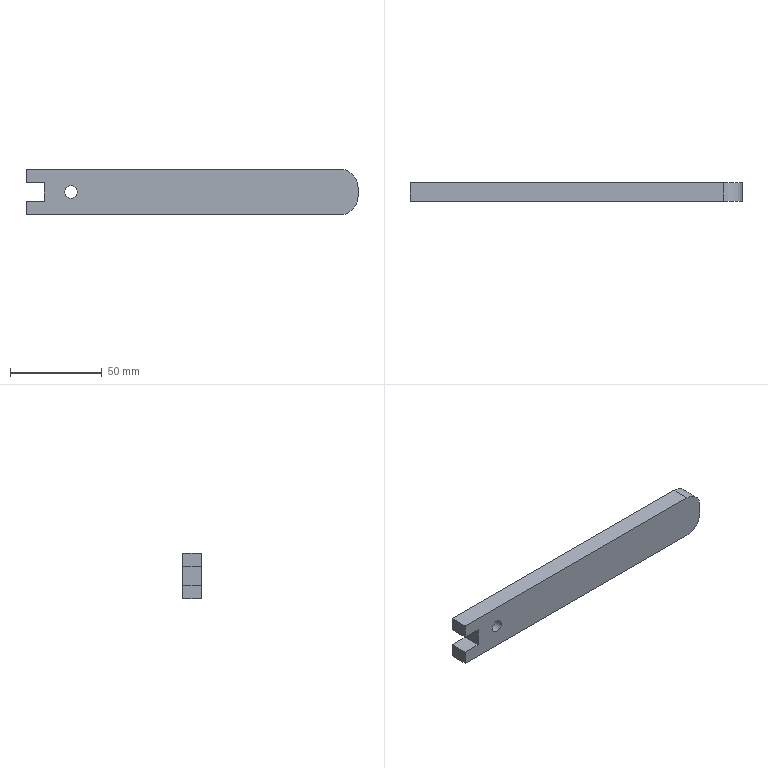Part | NX | features DATUM_CSYS 1, EXTRACT_DATUM_PLANE 1, EXTRUDE 1, SKETCH 1 | 1 solid | 13 faces | box 180.75 x 10 x 25 mm | volume 43395 mm3 | plane 10 | cylinder 3 | commonest cylinder face diameters 20 x2 6.8 x1
STEP:
#1=CARTESIAN_POINT('',(169.25,5.,17.214));
#2=VERTEX_POINT('',#1);
#3=CARTESIAN_POINT('',(169.25,5.,24.714));
#4=VERTEX_POINT('',#3);
#5=CARTESIAN_POINT('',(169.25,5.,17.214));
#6=DIRECTION('',(0.,0.,1.));
#7=VECTOR('',#6,1000.);
#8=LINE('',#5,#7);
#9=EDGE_CURVE('',#2,#4,#8,.T.);
#10=ORIENTED_EDGE('',*,*,#9,.F.);
#11=CARTESIAN_POINT('',(169.25,-5.,17.214));
#12=VERTEX_POINT('',#11);
#13=CARTESIAN_POINT('',(169.25,-5.,17.214));
#14=DIRECTION('',(0.,1.,0.));
#15=VECTOR('',#14,1000.);
#16=LINE('',#13,#15);
#17=EDGE_CURVE('',#12,#2,#16,.T.);
#18=ORIENTED_EDGE('',*,*,#17,.F.);
#19=CARTESIAN_POINT('',(169.25,-5.,24.714));
#20=VERTEX_POINT('',#19);
#21=CARTESIAN_POINT('',(169.25,-5.,17.214));
#22=DIRECTION('',(0.,0.,1.));
#23=VECTOR('',#22,1000.);
#24=LINE('',#21,#23);
#25=EDGE_CURVE('',#12,#20,#24,.T.);
#26=ORIENTED_EDGE('',*,*,#25,.T.);
#27=CARTESIAN_POINT('',(169.25,-5.,24.714));
#28=DIRECTION('',(0.,1.,0.));
#29=VECTOR('',#28,1000.);
#30=LINE('',#27,#29);
#31=EDGE_CURVE('',#20,#4,#30,.T.);
#32=ORIENTED_EDGE('',*,*,#31,.T.);
#33=EDGE_LOOP('',(#10,#18,#26,#32));
#34=FACE_BOUND('',#33,.T.);
#35=CARTESIAN_POINT('',(169.25,-5.,17.214));
#36=DIRECTION('',(-1.,0.,0.));
#37=DIRECTION('',(0.,0.,1.));
#38=AXIS2_PLACEMENT_3D('',#35,#36,#37);
#39=PLANE('',#38);
#40=ADVANCED_FACE('',(#34),#39,.T.);
#41=CARTESIAN_POINT('',(179.25,5.,24.714));
#42=VERTEX_POINT('',#41);
#43=CARTESIAN_POINT('',(174.25,5.,24.714));
#44=DIRECTION('',(1.,0.,0.));
#45=VECTOR('',#44,1000.);
#46=LINE('',#43,#45);
#47=EDGE_CURVE('',#4,#42,#46,.T.);
#48=ORIENTED_EDGE('',*,*,#47,.F.);
#49=ORIENTED_EDGE('',*,*,#31,.F.);
#50=CARTESIAN_POINT('',(179.25,-5.,24.714));
#51=VERTEX_POINT('',#50);
#52=CARTESIAN_POINT('',(169.25,-5.,24.714));
#53=DIRECTION('',(1.,0.,0.));
#54=VECTOR('',#53,1000.);
#55=LINE('',#52,#54);
#56=EDGE_CURVE('',#20,#51,#55,.T.);
#57=ORIENTED_EDGE('',*,*,#56,.T.);
#58=CARTESIAN_POINT('',(179.25,-5.,24.714));
#59=DIRECTION('',(0.,1.,0.));
#60=VECTOR('',#59,1000.);
#61=LINE('',#58,#60);
#62=EDGE_CURVE('',#51,#42,#61,.T.);
#63=ORIENTED_EDGE('',*,*,#62,.T.);
#64=EDGE_LOOP('',(#48,#49,#57,#63));
#65=FACE_BOUND('',#64,.T.);
#66=CARTESIAN_POINT('',(174.25,-5.,24.714));
#67=DIRECTION('',(0.,0.,1.));
#68=DIRECTION('',(1.,0.,0.));
#69=AXIS2_PLACEMENT_3D('',#66,#67,#68);
#70=PLANE('',#69);
#71=ADVANCED_FACE('',(#65),#70,.T.);
#72=CARTESIAN_POINT('',(179.25,5.,34.714));
#73=VERTEX_POINT('',#72);
#74=CARTESIAN_POINT('',(179.25,5.,24.714));
#75=DIRECTION('',(0.,0.,1.));
#76=VECTOR('',#75,1000.);
#77=LINE('',#74,#76);
#78=EDGE_CURVE('',#42,#73,#77,.T.);
#79=ORIENTED_EDGE('',*,*,#78,.F.);
#80=ORIENTED_EDGE('',*,*,#62,.F.);
#81=CARTESIAN_POINT('',(179.25,-5.,34.714));
#82=VERTEX_POINT('',#81);
#83=CARTESIAN_POINT('',(179.25,-5.,24.714));
#84=DIRECTION('',(0.,0.,1.));
#85=VECTOR('',#84,1000.);
#86=LINE('',#83,#85);
#87=EDGE_CURVE('',#51,#82,#86,.T.);
#88=ORIENTED_EDGE('',*,*,#87,.T.);
#89=CARTESIAN_POINT('',(179.25,-5.,34.714));
#90=DIRECTION('',(0.,1.,0.));
#91=VECTOR('',#90,1000.);
#92=LINE('',#89,#91);
#93=EDGE_CURVE('',#82,#73,#92,.T.);
#94=ORIENTED_EDGE('',*,*,#93,.T.);
#95=EDGE_LOOP('',(#79,#80,#88,#94));
#96=FACE_BOUND('',#95,.T.);
#97=CARTESIAN_POINT('',(179.25,-5.,24.714));
#98=DIRECTION('',(-1.,0.,0.));
#99=DIRECTION('',(0.,0.,1.));
#100=AXIS2_PLACEMENT_3D('',#97,#98,#99);
#101=PLANE('',#100);
#102=ADVANCED_FACE('',(#96),#101,.T.);
#103=CARTESIAN_POINT('',(169.25,5.,34.714));
#104=VERTEX_POINT('',#103);
#105=CARTESIAN_POINT('',(174.25,5.,34.714));
#106=DIRECTION('',(-1.,0.,0.));
#107=VECTOR('',#106,1000.);
#108=LINE('',#105,#107);
#109=EDGE_CURVE('',#73,#104,#108,.T.);
#110=ORIENTED_EDGE('',*,*,#109,.F.);
#111=ORIENTED_EDGE('',*,*,#93,.F.);
#112=CARTESIAN_POINT('',(169.25,-5.,34.714));
#113=VERTEX_POINT('',#112);
#114=CARTESIAN_POINT('',(179.25,-5.,34.714));
#115=DIRECTION('',(-1.,0.,0.));
#116=VECTOR('',#115,1000.);
#117=LINE('',#114,#116);
#118=EDGE_CURVE('',#82,#113,#117,.T.);
#119=ORIENTED_EDGE('',*,*,#118,.T.);
#120=CARTESIAN_POINT('',(169.25,-5.,34.714));
#121=DIRECTION('',(0.,1.,0.));
#122=VECTOR('',#121,1000.);
#123=LINE('',#120,#122);
#124=EDGE_CURVE('',#113,#104,#123,.T.);
#125=ORIENTED_EDGE('',*,*,#124,.T.);
#126=EDGE_LOOP('',(#110,#111,#119,#125));
#127=FACE_BOUND('',#126,.T.);
#128=CARTESIAN_POINT('',(174.25,-5.,34.714));
#129=DIRECTION('',(0.,0.,-1.));
#130=DIRECTION('',(-1.,0.,0.));
#131=AXIS2_PLACEMENT_3D('',#128,#129,#130);
#132=PLANE('',#131);
#133=ADVANCED_FACE('',(#127),#132,.T.);
#134=CARTESIAN_POINT('',(169.25,5.,42.214));
#135=VERTEX_POINT('',#134);
#136=CARTESIAN_POINT('',(169.25,5.,34.714));
#137=DIRECTION('',(0.,0.,1.));
#138=VECTOR('',#137,1000.);
#139=LINE('',#136,#138);
#140=EDGE_CURVE('',#104,#135,#139,.T.);
#141=ORIENTED_EDGE('',*,*,#140,.F.);
#142=ORIENTED_EDGE('',*,*,#124,.F.);
#143=CARTESIAN_POINT('',(169.25,-5.,42.214));
#144=VERTEX_POINT('',#143);
#145=CARTESIAN_POINT('',(169.25,-5.,34.714));
#146=DIRECTION('',(0.,0.,1.));
#147=VECTOR('',#146,1000.);
#148=LINE('',#145,#147);
#149=EDGE_CURVE('',#113,#144,#148,.T.);
#150=ORIENTED_EDGE('',*,*,#149,.T.);
#151=CARTESIAN_POINT('',(169.25,-5.,42.214));
#152=DIRECTION('',(0.,1.,0.));
#153=VECTOR('',#152,1000.);
#154=LINE('',#151,#153);
#155=EDGE_CURVE('',#144,#135,#154,.T.);
#156=ORIENTED_EDGE('',*,*,#155,.T.);
#157=EDGE_LOOP('',(#141,#142,#150,#156));
#158=FACE_BOUND('',#157,.T.);
#159=CARTESIAN_POINT('',(169.25,-5.,34.714));
#160=DIRECTION('',(-1.,0.,0.));
#161=DIRECTION('',(0.,0.,1.));
#162=AXIS2_PLACEMENT_3D('',#159,#160,#161);
#163=PLANE('',#162);
#164=ADVANCED_FACE('',(#158),#163,.T.);
#165=CARTESIAN_POINT('',(340.,5.,42.214));
#166=VERTEX_POINT('',#165);
#167=CARTESIAN_POINT('',(174.25,5.,42.214));
#168=DIRECTION('',(1.,0.,0.));
#169=VECTOR('',#168,1000.);
#170=LINE('',#167,#169);
#171=EDGE_CURVE('',#135,#166,#170,.T.);
#172=ORIENTED_EDGE('',*,*,#171,.F.);
#173=ORIENTED_EDGE('',*,*,#155,.F.);
#174=CARTESIAN_POINT('',(340.,-5.,42.214));
#175=VERTEX_POINT('',#174);
#176=CARTESIAN_POINT('',(169.25,-5.,42.214));
#177=DIRECTION('',(1.,0.,0.));
#178=VECTOR('',#177,1000.);
#179=LINE('',#176,#178);
#180=EDGE_CURVE('',#144,#175,#179,.T.);
#181=ORIENTED_EDGE('',*,*,#180,.T.);
#182=CARTESIAN_POINT('',(340.,-5.,42.214));
#183=DIRECTION('',(0.,1.,0.));
#184=VECTOR('',#183,1000.);
#185=LINE('',#182,#184);
#186=EDGE_CURVE('',#175,#166,#185,.T.);
#187=ORIENTED_EDGE('',*,*,#186,.T.);
#188=EDGE_LOOP('',(#172,#173,#181,#187));
#189=FACE_BOUND('',#188,.T.);
#190=CARTESIAN_POINT('',(174.25,-5.,42.214));
#191=DIRECTION('',(0.,0.,1.));
#192=DIRECTION('',(1.,0.,0.));
#193=AXIS2_PLACEMENT_3D('',#190,#191,#192);
#194=PLANE('',#193);
#195=ADVANCED_FACE('',(#189),#194,.T.);
#196=CARTESIAN_POINT('',(350.,5.,32.214));
#197=VERTEX_POINT('',#196);
#198=CARTESIAN_POINT('',(340.,5.,32.214));
#199=DIRECTION('',(0.,1.,0.));
#200=DIRECTION('',(0.,0.,1.));
#201=AXIS2_PLACEMENT_3D('',#198,#199,#200);
#202=CIRCLE('',#201,10.);
#203=EDGE_CURVE('',#166,#197,#202,.T.);
#204=ORIENTED_EDGE('',*,*,#203,.F.);
#205=ORIENTED_EDGE('',*,*,#186,.F.);
#206=CARTESIAN_POINT('',(350.,-5.,32.214));
#207=VERTEX_POINT('',#206);
#208=CARTESIAN_POINT('',(340.,-5.,32.214));
#209=DIRECTION('',(0.,1.,0.));
#210=DIRECTION('',(0.,0.,1.));
#211=AXIS2_PLACEMENT_3D('',#208,#209,#210);
#212=CIRCLE('',#211,10.);
#213=EDGE_CURVE('',#175,#207,#212,.T.);
#214=ORIENTED_EDGE('',*,*,#213,.T.);
#215=CARTESIAN_POINT('',(350.,-5.,32.214));
#216=DIRECTION('',(0.,1.,0.));
#217=VECTOR('',#216,1000.);
#218=LINE('',#215,#217);
#219=EDGE_CURVE('',#207,#197,#218,.T.);
#220=ORIENTED_EDGE('',*,*,#219,.T.);
#221=EDGE_LOOP('',(#204,#205,#214,#220));
#222=FACE_BOUND('',#221,.T.);
#223=CARTESIAN_POINT('',(340.,-5.,32.214));
#224=DIRECTION('',(0.,1.,0.));
#225=DIRECTION('',(0.,0.,1.));
#226=AXIS2_PLACEMENT_3D('',#223,#224,#225);
#227=CYLINDRICAL_SURFACE('',#226,10.);
#228=ADVANCED_FACE('',(#222),#227,.T.);
#229=CARTESIAN_POINT('',(350.,5.,27.214));
#230=VERTEX_POINT('',#229);
#231=CARTESIAN_POINT('',(350.,5.,32.214));
#232=DIRECTION('',(0.,0.,-1.));
#233=VECTOR('',#232,1000.);
#234=LINE('',#231,#233);
#235=EDGE_CURVE('',#197,#230,#234,.T.);
#236=ORIENTED_EDGE('',*,*,#235,.F.);
#237=ORIENTED_EDGE('',*,*,#219,.F.);
#238=CARTESIAN_POINT('',(350.,-5.,27.214));
#239=VERTEX_POINT('',#238);
#240=CARTESIAN_POINT('',(350.,-5.,32.214));
#241=DIRECTION('',(0.,0.,-1.));
#242=VECTOR('',#241,1000.);
#243=LINE('',#240,#242);
#244=EDGE_CURVE('',#207,#239,#243,.T.);
#245=ORIENTED_EDGE('',*,*,#244,.T.);
#246=CARTESIAN_POINT('',(350.,-5.,27.214));
#247=DIRECTION('',(0.,1.,0.));
#248=VECTOR('',#247,1000.);
#249=LINE('',#246,#248);
#250=EDGE_CURVE('',#239,#230,#249,.T.);
#251=ORIENTED_EDGE('',*,*,#250,.T.);
#252=EDGE_LOOP('',(#236,#237,#245,#251));
#253=FACE_BOUND('',#252,.T.);
#254=CARTESIAN_POINT('',(350.,-5.,32.214));
#255=DIRECTION('',(1.,0.,0.));
#256=DIRECTION('',(0.,0.,-1.));
#257=AXIS2_PLACEMENT_3D('',#254,#255,#256);
#258=PLANE('',#257);
#259=ADVANCED_FACE('',(#253),#258,.T.);
#260=CARTESIAN_POINT('',(340.,5.,17.214));
#261=VERTEX_POINT('',#260);
#262=CARTESIAN_POINT('',(340.,5.,27.214));
#263=DIRECTION('',(0.,1.,0.));
#264=DIRECTION('',(1.,0.,0.));
#265=AXIS2_PLACEMENT_3D('',#262,#263,#264);
#266=CIRCLE('',#265,10.);
#267=EDGE_CURVE('',#230,#261,#266,.T.);
#268=ORIENTED_EDGE('',*,*,#267,.F.);
#269=ORIENTED_EDGE('',*,*,#250,.F.);
#270=CARTESIAN_POINT('',(340.,-5.,17.214));
#271=VERTEX_POINT('',#270);
#272=CARTESIAN_POINT('',(340.,-5.,27.214));
#273=DIRECTION('',(0.,1.,0.));
#274=DIRECTION('',(1.,0.,0.));
#275=AXIS2_PLACEMENT_3D('',#272,#273,#274);
#276=CIRCLE('',#275,10.);
#277=EDGE_CURVE('',#239,#271,#276,.T.);
#278=ORIENTED_EDGE('',*,*,#277,.T.);
#279=CARTESIAN_POINT('',(340.,-5.,17.214));
#280=DIRECTION('',(0.,1.,0.));
#281=VECTOR('',#280,1000.);
#282=LINE('',#279,#281);
#283=EDGE_CURVE('',#271,#261,#282,.T.);
#284=ORIENTED_EDGE('',*,*,#283,.T.);
#285=EDGE_LOOP('',(#268,#269,#278,#284));
#286=FACE_BOUND('',#285,.T.);
#287=CARTESIAN_POINT('',(340.,-5.,27.214));
#288=DIRECTION('',(0.,1.,0.));
#289=DIRECTION('',(0.,0.,1.));
#290=AXIS2_PLACEMENT_3D('',#287,#288,#289);
#291=CYLINDRICAL_SURFACE('',#290,10.);
#292=ADVANCED_FACE('',(#286),#291,.T.);
#293=CARTESIAN_POINT('',(174.25,5.,17.214));
#294=DIRECTION('',(-1.,0.,0.));
#295=VECTOR('',#294,1000.);
#296=LINE('',#293,#295);
#297=EDGE_CURVE('',#261,#2,#296,.T.);
#298=ORIENTED_EDGE('',*,*,#297,.F.);
#299=ORIENTED_EDGE('',*,*,#283,.F.);
#300=CARTESIAN_POINT('',(340.,-5.,17.214));
#301=DIRECTION('',(-1.,0.,0.));
#302=VECTOR('',#301,1000.);
#303=LINE('',#300,#302);
#304=EDGE_CURVE('',#271,#12,#303,.T.);
#305=ORIENTED_EDGE('',*,*,#304,.T.);
#306=ORIENTED_EDGE('',*,*,#17,.T.);
#307=EDGE_LOOP('',(#298,#299,#305,#306));
#308=FACE_BOUND('',#307,.T.);
#309=CARTESIAN_POINT('',(174.25,-5.,17.214));
#310=DIRECTION('',(0.,0.,-1.));
#311=DIRECTION('',(-1.,0.,0.));
#312=AXIS2_PLACEMENT_3D('',#309,#310,#311);
#313=PLANE('',#312);
#314=ADVANCED_FACE('',(#308),#313,.T.);
#315=CARTESIAN_POINT('',(193.75,5.,26.314));
#316=VERTEX_POINT('',#315);
#317=CARTESIAN_POINT('',(193.75,5.,29.714));
#318=DIRECTION('',(0.,-1.,0.));
#319=DIRECTION('',(0.,0.,-1.));
#320=AXIS2_PLACEMENT_3D('',#317,#318,#319);
#321=CIRCLE('',#320,3.4);
#322=EDGE_CURVE('',#316,#316,#321,.T.);
#323=ORIENTED_EDGE('',*,*,#322,.F.);
#324=EDGE_LOOP('',(#323));
#325=FACE_BOUND('',#324,.T.);
#326=CARTESIAN_POINT('',(193.75,-5.,33.114));
#327=VERTEX_POINT('',#326);
#328=CARTESIAN_POINT('',(193.75,-5.,29.714));
#329=DIRECTION('',(0.,-1.,0.));
#330=DIRECTION('',(0.,0.,1.));
#331=AXIS2_PLACEMENT_3D('',#328,#329,#330);
#332=CIRCLE('',#331,3.4);
#333=EDGE_CURVE('',#327,#327,#332,.T.);
#334=ORIENTED_EDGE('',*,*,#333,.T.);
#335=EDGE_LOOP('',(#334));
#336=FACE_BOUND('',#335,.T.);
#337=CARTESIAN_POINT('',(193.75,-5.,29.714));
#338=DIRECTION('',(0.,1.,0.));
#339=DIRECTION('',(0.,0.,1.));
#340=AXIS2_PLACEMENT_3D('',#337,#338,#339);
#341=CYLINDRICAL_SURFACE('',#340,3.4);
#342=ADVANCED_FACE('',(#325,#336),#341,.F.);
#343=ORIENTED_EDGE('',*,*,#25,.F.);
#344=ORIENTED_EDGE('',*,*,#304,.F.);
#345=ORIENTED_EDGE('',*,*,#277,.F.);
#346=ORIENTED_EDGE('',*,*,#244,.F.);
#347=ORIENTED_EDGE('',*,*,#213,.F.);
#348=ORIENTED_EDGE('',*,*,#180,.F.);
#349=ORIENTED_EDGE('',*,*,#149,.F.);
#350=ORIENTED_EDGE('',*,*,#118,.F.);
#351=ORIENTED_EDGE('',*,*,#87,.F.);
#352=ORIENTED_EDGE('',*,*,#56,.F.);
#353=EDGE_LOOP('',(#343,#344,#345,#346,#347,#348,#349,#350,#351,#352));
#354=FACE_BOUND('',#353,.T.);
#355=ORIENTED_EDGE('',*,*,#333,.F.);
#356=EDGE_LOOP('',(#355));
#357=FACE_BOUND('',#356,.T.);
#358=CARTESIAN_POINT('',(340.,-5.,32.214));
#359=DIRECTION('',(0.,1.,0.));
#360=DIRECTION('',(0.,0.,1.));
#361=AXIS2_PLACEMENT_3D('',#358,#359,#360);
#362=PLANE('',#361);
#363=ADVANCED_FACE('',(#354,#357),#362,.F.);
#364=ORIENTED_EDGE('',*,*,#9,.T.);
#365=ORIENTED_EDGE('',*,*,#47,.T.);
#366=ORIENTED_EDGE('',*,*,#78,.T.);
#367=ORIENTED_EDGE('',*,*,#109,.T.);
#368=ORIENTED_EDGE('',*,*,#140,.T.);
#369=ORIENTED_EDGE('',*,*,#171,.T.);
#370=ORIENTED_EDGE('',*,*,#203,.T.);
#371=ORIENTED_EDGE('',*,*,#235,.T.);
#372=ORIENTED_EDGE('',*,*,#267,.T.);
#373=ORIENTED_EDGE('',*,*,#297,.T.);
#374=EDGE_LOOP('',(#364,#365,#366,#367,#368,#369,#370,#371,#372,#373));
#375=FACE_BOUND('',#374,.T.);
#376=ORIENTED_EDGE('',*,*,#322,.T.);
#377=EDGE_LOOP('',(#376));
#378=FACE_BOUND('',#377,.T.);
#379=CARTESIAN_POINT('',(340.,5.,32.214));
#380=DIRECTION('',(0.,1.,0.));
#381=DIRECTION('',(0.,0.,1.));
#382=AXIS2_PLACEMENT_3D('',#379,#380,#381);
#383=PLANE('',#382);
#384=ADVANCED_FACE('',(#375,#378),#383,.T.);
#385=CLOSED_SHELL('',(#40,#71,#102,#133,#164,#195,#228,#259,#292,#314,#342,#363,#384));
#386=MANIFOLD_SOLID_BREP('',#385);
#387=(LENGTH_UNIT()NAMED_UNIT(*)SI_UNIT(.MILLI.,.METRE.));
#388=UNCERTAINTY_MEASURE_WITH_UNIT(LENGTH_MEASURE(0.00001),#387,'','');
#389=(NAMED_UNIT(*)PLANE_ANGLE_UNIT()SI_UNIT($,.RADIAN.));
#390=(NAMED_UNIT(*)SI_UNIT($,.STERADIAN.)SOLID_ANGLE_UNIT());
#391=(GEOMETRIC_REPRESENTATION_CONTEXT(3)GLOBAL_UNCERTAINTY_ASSIGNED_CONTEXT((#388))GLOBAL_UNIT_ASSIGNED_CONTEXT((#387,#389,#390))REPRESENTATION_CONTEXT('',''));
#392=ADVANCED_BREP_SHAPE_REPRESENTATION('',(#386),#391);